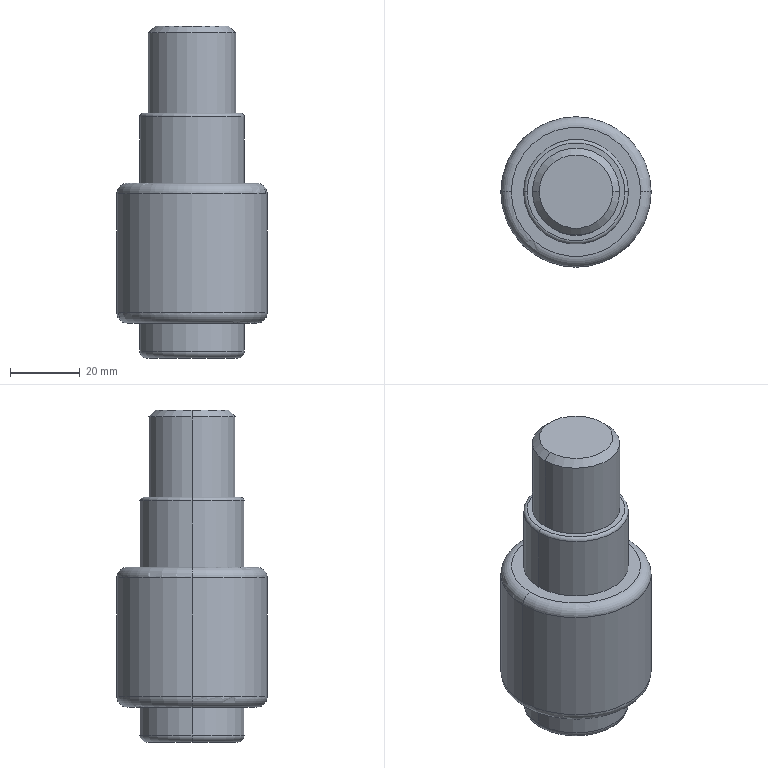Part | STEP file | Blocking air bag | 1 solid | 23 faces | box 43 x 43 x 95 mm | volume 90813 mm3 | torus 8 | cylinder 8 | plane 5 | cone 2 | commonest cylinder face diameters 30 x4 25 x2 43 x2
STEP:
#1=CARTESIAN_POINT('',(0.,0.,0.));
#2=DIRECTION('',(0.,0.,1.));
#3=DIRECTION('',(1.,0.,0.));
#4=AXIS2_PLACEMENT_3D('',#1,#2,#3);
#5=CARTESIAN_POINT('',(10.5,0.,95.));
#6=VERTEX_POINT('',#5);
#7=CARTESIAN_POINT('',(-10.5,0.,95.));
#8=VERTEX_POINT('',#7);
#9=CARTESIAN_POINT('',(0.,0.,95.));
#10=DIRECTION('',(0.,0.,1.));
#11=DIRECTION('',(1.,0.,0.));
#12=AXIS2_PLACEMENT_3D('',#9,#10,#11);
#13=CIRCLE('',#12,10.5);
#14=CARTESIAN_POINT('',(0.,0.,95.));
#15=DIRECTION('',(0.,0.,-1.));
#16=DIRECTION('',(-1.,0.,0.));
#17=AXIS2_PLACEMENT_3D('',#14,#15,#16);
#18=CONICAL_SURFACE('',#17,10.5,0.7854);
#19=CARTESIAN_POINT('',(3.142,0.));
#20=DIRECTION('',(-1.,0.));
#21=VECTOR('',#20,1.);
#22=LINE('',#19,#21);
#23=(GEOMETRIC_REPRESENTATION_CONTEXT(2)PARAMETRIC_REPRESENTATION_CONTEXT()REPRESENTATION_CONTEXT('',''));
#24=DEFINITIONAL_REPRESENTATION('',(#22),#23);
#25=PCURVE('',#18,#24);
#26=CARTESIAN_POINT('',(12.5,0.,95.));
#27=DIRECTION('',(0.,0.,1.));
#28=DIRECTION('',(1.,0.,0.));
#29=AXIS2_PLACEMENT_3D('',#26,#27,#28);
#30=PLANE('',#29);
#31=CARTESIAN_POINT('',(-12.5,0.));
#32=DIRECTION('',(1.,0.));
#33=AXIS2_PLACEMENT_2D('',#31,#32);
#34=CIRCLE('',#33,10.5);
#35=(GEOMETRIC_REPRESENTATION_CONTEXT(2)PARAMETRIC_REPRESENTATION_CONTEXT()REPRESENTATION_CONTEXT('',''));
#36=DEFINITIONAL_REPRESENTATION('',(#34),#35);
#37=PCURVE('',#30,#36);
#38=SURFACE_CURVE('',#13,(#25,#37),.PCURVE_S1.);
#39=EDGE_CURVE('',#6,#8,#38,.T.);
#40=ORIENTED_EDGE('',*,*,#39,.F.);
#41=CARTESIAN_POINT('',(12.5,0.,93.));
#42=VERTEX_POINT('',#41);
#43=CARTESIAN_POINT('',(10.5,0.,95.));
#44=DIRECTION('',(0.7071,0.,-0.7071));
#45=VECTOR('',#44,1.);
#46=LINE('',#43,#45);
#47=CARTESIAN_POINT('',(3.142,0.));
#48=DIRECTION('',(0.,1.));
#49=VECTOR('',#48,1.);
#50=LINE('',#47,#49);
#51=(GEOMETRIC_REPRESENTATION_CONTEXT(2)PARAMETRIC_REPRESENTATION_CONTEXT()REPRESENTATION_CONTEXT('',''));
#52=DEFINITIONAL_REPRESENTATION('',(#50),#51);
#53=PCURVE('',#18,#52);
#54=CARTESIAN_POINT('',(0.,0.,95.));
#55=DIRECTION('',(0.,0.,-1.));
#56=DIRECTION('',(-1.,0.,0.));
#57=AXIS2_PLACEMENT_3D('',#54,#55,#56);
#58=CONICAL_SURFACE('',#57,10.5,0.7854);
#59=CARTESIAN_POINT('',(3.142,0.));
#60=DIRECTION('',(0.,1.));
#61=VECTOR('',#60,1.);
#62=LINE('',#59,#61);
#63=(GEOMETRIC_REPRESENTATION_CONTEXT(2)PARAMETRIC_REPRESENTATION_CONTEXT()REPRESENTATION_CONTEXT('',''));
#64=DEFINITIONAL_REPRESENTATION('',(#62),#63);
#65=PCURVE('',#58,#64);
#66=SURFACE_CURVE('',#46,(#53,#65),.PCURVE_S1.);
#67=EDGE_CURVE('',#6,#42,#66,.T.);
#68=ORIENTED_EDGE('',*,*,#67,.T.);
#69=CARTESIAN_POINT('',(-12.5,0.,93.));
#70=VERTEX_POINT('',#69);
#71=CARTESIAN_POINT('',(0.,0.,93.));
#72=DIRECTION('',(0.,0.,-1.));
#73=DIRECTION('',(1.,0.,0.));
#74=AXIS2_PLACEMENT_3D('',#71,#72,#73);
#75=CIRCLE('',#74,12.5);
#76=CARTESIAN_POINT('',(-3.142,2.));
#77=DIRECTION('',(1.,0.));
#78=VECTOR('',#77,1.);
#79=LINE('',#76,#78);
#80=(GEOMETRIC_REPRESENTATION_CONTEXT(2)PARAMETRIC_REPRESENTATION_CONTEXT()REPRESENTATION_CONTEXT('',''));
#81=DEFINITIONAL_REPRESENTATION('',(#79),#80);
#82=PCURVE('',#18,#81);
#83=CARTESIAN_POINT('',(0.,0.,95.));
#84=DIRECTION('',(0.,0.,1.));
#85=DIRECTION('',(1.,0.,0.));
#86=AXIS2_PLACEMENT_3D('',#83,#84,#85);
#87=CYLINDRICAL_SURFACE('',#86,12.5);
#88=CARTESIAN_POINT('',(6.283,-2.));
#89=DIRECTION('',(-1.,0.));
#90=VECTOR('',#89,1.);
#91=LINE('',#88,#90);
#92=(GEOMETRIC_REPRESENTATION_CONTEXT(2)PARAMETRIC_REPRESENTATION_CONTEXT()REPRESENTATION_CONTEXT('',''));
#93=DEFINITIONAL_REPRESENTATION('',(#91),#92);
#94=PCURVE('',#87,#93);
#95=SURFACE_CURVE('',#75,(#82,#94),.PCURVE_S1.);
#96=EDGE_CURVE('',#70,#42,#95,.T.);
#97=ORIENTED_EDGE('',*,*,#96,.F.);
#98=CARTESIAN_POINT('',(-10.5,0.,95.));
#99=DIRECTION('',(-0.7071,0.,-0.7071));
#100=VECTOR('',#99,1.);
#101=LINE('',#98,#100);
#102=CARTESIAN_POINT('',(0.,0.));
#103=DIRECTION('',(0.,1.));
#104=VECTOR('',#103,1.);
#105=LINE('',#102,#104);
#106=(GEOMETRIC_REPRESENTATION_CONTEXT(2)PARAMETRIC_REPRESENTATION_CONTEXT()REPRESENTATION_CONTEXT('',''));
#107=DEFINITIONAL_REPRESENTATION('',(#105),#106);
#108=PCURVE('',#18,#107);
#109=CARTESIAN_POINT('',(6.283,0.));
#110=DIRECTION('',(0.,1.));
#111=VECTOR('',#110,1.);
#112=LINE('',#109,#111);
#113=(GEOMETRIC_REPRESENTATION_CONTEXT(2)PARAMETRIC_REPRESENTATION_CONTEXT()REPRESENTATION_CONTEXT('',''));
#114=DEFINITIONAL_REPRESENTATION('',(#112),#113);
#115=PCURVE('',#58,#114);
#116=SURFACE_CURVE('',#101,(#108,#115),.PCURVE_S1.);
#117=EDGE_CURVE('',#8,#70,#116,.T.);
#118=ORIENTED_EDGE('',*,*,#117,.F.);
#119=EDGE_LOOP('',(#40,#68,#97,#118));
#120=FACE_BOUND('',#119,.T.);
#121=ADVANCED_FACE('',(#120),#18,.T.);
#122=CARTESIAN_POINT('',(15.,0.,2.));
#123=VERTEX_POINT('',#122);
#124=CARTESIAN_POINT('',(-15.,0.,2.));
#125=VERTEX_POINT('',#124);
#126=CARTESIAN_POINT('',(0.,0.,2.));
#127=DIRECTION('',(0.,0.,1.));
#128=DIRECTION('',(-1.,0.,0.));
#129=AXIS2_PLACEMENT_3D('',#126,#127,#128);
#130=CIRCLE('',#129,15.);
#131=CARTESIAN_POINT('',(0.,0.,2.));
#132=DIRECTION('',(0.,0.,-1.));
#133=DIRECTION('',(-1.,0.,0.));
#134=AXIS2_PLACEMENT_3D('',#131,#132,#133);
#135=TOROIDAL_SURFACE('',#134,13.,2.);
#136=CARTESIAN_POINT('',(6.283,0.));
#137=DIRECTION('',(-1.,0.));
#138=VECTOR('',#137,1.);
#139=LINE('',#136,#138);
#140=(GEOMETRIC_REPRESENTATION_CONTEXT(2)PARAMETRIC_REPRESENTATION_CONTEXT()REPRESENTATION_CONTEXT('',''));
#141=DEFINITIONAL_REPRESENTATION('',(#139),#140);
#142=PCURVE('',#135,#141);
#143=CARTESIAN_POINT('',(0.,0.,95.));
#144=DIRECTION('',(0.,0.,1.));
#145=DIRECTION('',(1.,0.,0.));
#146=AXIS2_PLACEMENT_3D('',#143,#144,#145);
#147=CYLINDRICAL_SURFACE('',#146,15.);
#148=CARTESIAN_POINT('',(-3.142,-93.));
#149=DIRECTION('',(1.,0.));
#150=VECTOR('',#149,1.);
#151=LINE('',#148,#150);
#152=(GEOMETRIC_REPRESENTATION_CONTEXT(2)PARAMETRIC_REPRESENTATION_CONTEXT()REPRESENTATION_CONTEXT('',''));
#153=DEFINITIONAL_REPRESENTATION('',(#151),#152);
#154=PCURVE('',#147,#153);
#155=SURFACE_CURVE('',#130,(#142,#154),.PCURVE_S1.);
#156=EDGE_CURVE('',#123,#125,#155,.T.);
#157=ORIENTED_EDGE('',*,*,#156,.F.);
#158=CARTESIAN_POINT('',(13.,0.,0.));
#159=VERTEX_POINT('',#158);
#160=CARTESIAN_POINT('',(13.,0.,2.));
#161=DIRECTION('',(0.,1.,0.));
#162=DIRECTION('',(-1.,0.,0.));
#163=AXIS2_PLACEMENT_3D('',#160,#161,#162);
#164=CIRCLE('',#163,2.);
#165=CARTESIAN_POINT('',(3.142,-3.142));
#166=DIRECTION('',(0.,1.));
#167=VECTOR('',#166,1.);
#168=LINE('',#165,#167);
#169=(GEOMETRIC_REPRESENTATION_CONTEXT(2)PARAMETRIC_REPRESENTATION_CONTEXT()REPRESENTATION_CONTEXT('',''));
#170=DEFINITIONAL_REPRESENTATION('',(#168),#169);
#171=PCURVE('',#135,#170);
#172=CARTESIAN_POINT('',(0.,0.,2.));
#173=DIRECTION('',(0.,0.,-1.));
#174=DIRECTION('',(-1.,0.,0.));
#175=AXIS2_PLACEMENT_3D('',#172,#173,#174);
#176=TOROIDAL_SURFACE('',#175,13.,2.);
#177=CARTESIAN_POINT('',(3.142,-3.142));
#178=DIRECTION('',(0.,1.));
#179=VECTOR('',#178,1.);
#180=LINE('',#177,#179);
#181=(GEOMETRIC_REPRESENTATION_CONTEXT(2)PARAMETRIC_REPRESENTATION_CONTEXT()REPRESENTATION_CONTEXT('',''));
#182=DEFINITIONAL_REPRESENTATION('',(#180),#181);
#183=PCURVE('',#176,#182);
#184=SURFACE_CURVE('',#164,(#171,#183),.PCURVE_S1.);
#185=EDGE_CURVE('',#123,#159,#184,.T.);
#186=ORIENTED_EDGE('',*,*,#185,.T.);
#187=CARTESIAN_POINT('',(-13.,0.,0.));
#188=VERTEX_POINT('',#187);
#189=CARTESIAN_POINT('',(0.,0.,0.));
#190=DIRECTION('',(0.,0.,-1.));
#191=DIRECTION('',(-1.,0.,0.));
#192=AXIS2_PLACEMENT_3D('',#189,#190,#191);
#193=CIRCLE('',#192,13.);
#194=CARTESIAN_POINT('',(0.,1.571));
#195=DIRECTION('',(1.,0.));
#196=VECTOR('',#195,1.);
#197=LINE('',#194,#196);
#198=(GEOMETRIC_REPRESENTATION_CONTEXT(2)PARAMETRIC_REPRESENTATION_CONTEXT()REPRESENTATION_CONTEXT('',''));
#199=DEFINITIONAL_REPRESENTATION('',(#197),#198);
#200=PCURVE('',#135,#199);
#201=CARTESIAN_POINT('',(0.,0.,0.));
#202=DIRECTION('',(0.,0.,-1.));
#203=DIRECTION('',(-1.,0.,0.));
#204=AXIS2_PLACEMENT_3D('',#201,#202,#203);
#205=PLANE('',#204);
#206=CARTESIAN_POINT('',(0.,0.));
#207=DIRECTION('',(1.,0.));
#208=AXIS2_PLACEMENT_2D('',#206,#207);
#209=CIRCLE('',#208,13.);
#210=(GEOMETRIC_REPRESENTATION_CONTEXT(2)PARAMETRIC_REPRESENTATION_CONTEXT()REPRESENTATION_CONTEXT('',''));
#211=DEFINITIONAL_REPRESENTATION('',(#209),#210);
#212=PCURVE('',#205,#211);
#213=SURFACE_CURVE('',#193,(#200,#212),.PCURVE_S1.);
#214=EDGE_CURVE('',#188,#159,#213,.T.);
#215=ORIENTED_EDGE('',*,*,#214,.F.);
#216=CARTESIAN_POINT('',(-13.,0.,2.));
#217=DIRECTION('',(0.,-1.,0.));
#218=DIRECTION('',(0.,0.,-1.));
#219=AXIS2_PLACEMENT_3D('',#216,#217,#218);
#220=CIRCLE('',#219,2.);
#221=CARTESIAN_POINT('',(0.,-4.712));
#222=DIRECTION('',(0.,1.));
#223=VECTOR('',#222,1.);
#224=LINE('',#221,#223);
#225=(GEOMETRIC_REPRESENTATION_CONTEXT(2)PARAMETRIC_REPRESENTATION_CONTEXT()REPRESENTATION_CONTEXT('',''));
#226=DEFINITIONAL_REPRESENTATION('',(#224),#225);
#227=PCURVE('',#135,#226);
#228=CARTESIAN_POINT('',(6.283,-4.712));
#229=DIRECTION('',(0.,1.));
#230=VECTOR('',#229,1.);
#231=LINE('',#228,#230);
#232=(GEOMETRIC_REPRESENTATION_CONTEXT(2)PARAMETRIC_REPRESENTATION_CONTEXT()REPRESENTATION_CONTEXT('',''));
#233=DEFINITIONAL_REPRESENTATION('',(#231),#232);
#234=PCURVE('',#176,#233);
#235=SURFACE_CURVE('',#220,(#227,#234),.PCURVE_S1.);
#236=EDGE_CURVE('',#125,#188,#235,.T.);
#237=ORIENTED_EDGE('',*,*,#236,.F.);
#238=EDGE_LOOP('',(#157,#186,#215,#237));
#239=FACE_BOUND('',#238,.T.);
#240=ADVANCED_FACE('',(#239),#135,.T.);
#241=CARTESIAN_POINT('',(-15.,0.,69.));
#242=VERTEX_POINT('',#241);
#243=CARTESIAN_POINT('',(15.,0.,69.));
#244=VERTEX_POINT('',#243);
#245=CARTESIAN_POINT('',(0.,0.,69.));
#246=DIRECTION('',(0.,0.,-1.));
#247=DIRECTION('',(1.,0.,0.));
#248=AXIS2_PLACEMENT_3D('',#245,#246,#247);
#249=CIRCLE('',#248,15.);
#250=CARTESIAN_POINT('',(0.,0.,69.));
#251=DIRECTION('',(0.,0.,1.));
#252=DIRECTION('',(1.,0.,0.));
#253=AXIS2_PLACEMENT_3D('',#250,#251,#252);
#254=TOROIDAL_SURFACE('',#253,14.,1.);
#255=CARTESIAN_POINT('',(6.283,0.));
#256=DIRECTION('',(-1.,0.));
#257=VECTOR('',#256,1.);
#258=LINE('',#255,#257);
#259=(GEOMETRIC_REPRESENTATION_CONTEXT(2)PARAMETRIC_REPRESENTATION_CONTEXT()REPRESENTATION_CONTEXT('',''));
#260=DEFINITIONAL_REPRESENTATION('',(#258),#259);
#261=PCURVE('',#254,#260);
#262=CARTESIAN_POINT('',(0.,0.,95.));
#263=DIRECTION('',(0.,0.,1.));
#264=DIRECTION('',(1.,0.,0.));
#265=AXIS2_PLACEMENT_3D('',#262,#263,#264);
#266=CYLINDRICAL_SURFACE('',#265,15.);
#267=CARTESIAN_POINT('',(6.283,-26.));
#268=DIRECTION('',(-1.,0.));
#269=VECTOR('',#268,1.);
#270=LINE('',#267,#269);
#271=(GEOMETRIC_REPRESENTATION_CONTEXT(2)PARAMETRIC_REPRESENTATION_CONTEXT()REPRESENTATION_CONTEXT('',''));
#272=DEFINITIONAL_REPRESENTATION('',(#270),#271);
#273=PCURVE('',#266,#272);
#274=SURFACE_CURVE('',#249,(#261,#273),.PCURVE_S1.);
#275=EDGE_CURVE('',#242,#244,#274,.T.);
#276=ORIENTED_EDGE('',*,*,#275,.F.);
#277=CARTESIAN_POINT('',(-14.,0.,70.));
#278=VERTEX_POINT('',#277);
#279=CARTESIAN_POINT('',(-14.,0.,69.));
#280=DIRECTION('',(0.,1.,0.));
#281=DIRECTION('',(-1.,0.,0.));
#282=AXIS2_PLACEMENT_3D('',#279,#280,#281);
#283=CIRCLE('',#282,1.);
#284=CARTESIAN_POINT('',(3.142,0.));
#285=DIRECTION('',(0.,1.));
#286=VECTOR('',#285,1.);
#287=LINE('',#284,#286);
#288=(GEOMETRIC_REPRESENTATION_CONTEXT(2)PARAMETRIC_REPRESENTATION_CONTEXT()REPRESENTATION_CONTEXT('',''));
#289=DEFINITIONAL_REPRESENTATION('',(#287),#288);
#290=PCURVE('',#254,#289);
#291=CARTESIAN_POINT('',(0.,0.,69.));
#292=DIRECTION('',(0.,0.,1.));
#293=DIRECTION('',(1.,0.,0.));
#294=AXIS2_PLACEMENT_3D('',#291,#292,#293);
#295=TOROIDAL_SURFACE('',#294,14.,1.);
#296=CARTESIAN_POINT('',(3.142,0.));
#297=DIRECTION('',(0.,1.));
#298=VECTOR('',#297,1.);
#299=LINE('',#296,#298);
#300=(GEOMETRIC_REPRESENTATION_CONTEXT(2)PARAMETRIC_REPRESENTATION_CONTEXT()REPRESENTATION_CONTEXT('',''));
#301=DEFINITIONAL_REPRESENTATION('',(#299),#300);
#302=PCURVE('',#295,#301);
#303=SURFACE_CURVE('',#283,(#290,#302),.PCURVE_S1.);
#304=EDGE_CURVE('',#242,#278,#303,.T.);
#305=ORIENTED_EDGE('',*,*,#304,.T.);
#306=CARTESIAN_POINT('',(14.,0.,70.));
#307=VERTEX_POINT('',#306);
#308=CARTESIAN_POINT('',(0.,0.,70.));
#309=DIRECTION('',(0.,0.,1.));
#310=DIRECTION('',(1.,0.,0.));
#311=AXIS2_PLACEMENT_3D('',#308,#309,#310);
#312=CIRCLE('',#311,14.);
#313=CARTESIAN_POINT('',(0.,1.571));
#314=DIRECTION('',(1.,0.));
#315=VECTOR('',#314,1.);
#316=LINE('',#313,#315);
#317=(GEOMETRIC_REPRESENTATION_CONTEXT(2)PARAMETRIC_REPRESENTATION_CONTEXT()REPRESENTATION_CONTEXT('',''));
#318=DEFINITIONAL_REPRESENTATION('',(#316),#317);
#319=PCURVE('',#254,#318);
#320=CARTESIAN_POINT('',(15.,0.,70.));
#321=DIRECTION('',(0.,0.,1.));
#322=DIRECTION('',(1.,0.,0.));
#323=AXIS2_PLACEMENT_3D('',#320,#321,#322);
#324=PLANE('',#323);
#325=CARTESIAN_POINT('',(-15.,0.));
#326=DIRECTION('',(1.,0.));
#327=AXIS2_PLACEMENT_2D('',#325,#326);
#328=CIRCLE('',#327,14.);
#329=(GEOMETRIC_REPRESENTATION_CONTEXT(2)PARAMETRIC_REPRESENTATION_CONTEXT()REPRESENTATION_CONTEXT('',''));
#330=DEFINITIONAL_REPRESENTATION('',(#328),#329);
#331=PCURVE('',#324,#330);
#332=SURFACE_CURVE('',#312,(#319,#331),.PCURVE_S1.);
#333=EDGE_CURVE('',#307,#278,#332,.T.);
#334=ORIENTED_EDGE('',*,*,#333,.F.);
#335=CARTESIAN_POINT('',(14.,0.,69.));
#336=DIRECTION('',(0.,-1.,0.));
#337=DIRECTION('',(0.,0.,-1.));
#338=AXIS2_PLACEMENT_3D('',#335,#336,#337);
#339=CIRCLE('',#338,1.);
#340=CARTESIAN_POINT('',(0.,-1.571));
#341=DIRECTION('',(0.,1.));
#342=VECTOR('',#341,1.);
#343=LINE('',#340,#342);
#344=(GEOMETRIC_REPRESENTATION_CONTEXT(2)PARAMETRIC_REPRESENTATION_CONTEXT()REPRESENTATION_CONTEXT('',''));
#345=DEFINITIONAL_REPRESENTATION('',(#343),#344);
#346=PCURVE('',#254,#345);
#347=CARTESIAN_POINT('',(6.283,-1.571));
#348=DIRECTION('',(0.,1.));
#349=VECTOR('',#348,1.);
#350=LINE('',#347,#349);
#351=(GEOMETRIC_REPRESENTATION_CONTEXT(2)PARAMETRIC_REPRESENTATION_CONTEXT()REPRESENTATION_CONTEXT('',''));
#352=DEFINITIONAL_REPRESENTATION('',(#350),#351);
#353=PCURVE('',#295,#352);
#354=SURFACE_CURVE('',#339,(#346,#353),.PCURVE_S1.);
#355=EDGE_CURVE('',#244,#307,#354,.T.);
#356=ORIENTED_EDGE('',*,*,#355,.F.);
#357=EDGE_LOOP('',(#276,#305,#334,#356));
#358=FACE_BOUND('',#357,.T.);
#359=ADVANCED_FACE('',(#358),#254,.T.);
#360=CARTESIAN_POINT('',(21.5,0.,13.));
#361=VERTEX_POINT('',#360);
#362=CARTESIAN_POINT('',(-21.5,0.,13.));
#363=VERTEX_POINT('',#362);
#364=CARTESIAN_POINT('',(0.,0.,13.));
#365=DIRECTION('',(0.,0.,1.));
#366=DIRECTION('',(-1.,0.,0.));
#367=AXIS2_PLACEMENT_3D('',#364,#365,#366);
#368=CIRCLE('',#367,21.5);
#369=CARTESIAN_POINT('',(0.,0.,13.));
#370=DIRECTION('',(0.,0.,-1.));
#371=DIRECTION('',(-1.,0.,0.));
#372=AXIS2_PLACEMENT_3D('',#369,#370,#371);
#373=TOROIDAL_SURFACE('',#372,18.5,3.);
#374=CARTESIAN_POINT('',(6.283,0.));
#375=DIRECTION('',(-1.,0.));
#376=VECTOR('',#375,1.);
#377=LINE('',#374,#376);
#378=(GEOMETRIC_REPRESENTATION_CONTEXT(2)PARAMETRIC_REPRESENTATION_CONTEXT()REPRESENTATION_CONTEXT('',''));
#379=DEFINITIONAL_REPRESENTATION('',(#377),#378);
#380=PCURVE('',#373,#379);
#381=CARTESIAN_POINT('',(0.,0.,95.));
#382=DIRECTION('',(0.,0.,1.));
#383=DIRECTION('',(1.,0.,0.));
#384=AXIS2_PLACEMENT_3D('',#381,#382,#383);
#385=CYLINDRICAL_SURFACE('',#384,21.5);
#386=CARTESIAN_POINT('',(-3.142,-82.));
#387=DIRECTION('',(1.,0.));
#388=VECTOR('',#387,1.);
#389=LINE('',#386,#388);
#390=(GEOMETRIC_REPRESENTATION_CONTEXT(2)PARAMETRIC_REPRESENTATION_CONTEXT()REPRESENTATION_CONTEXT('',''));
#391=DEFINITIONAL_REPRESENTATION('',(#389),#390);
#392=PCURVE('',#385,#391);
#393=SURFACE_CURVE('',#368,(#380,#392),.PCURVE_S1.);
#394=EDGE_CURVE('',#361,#363,#393,.T.);
#395=ORIENTED_EDGE('',*,*,#394,.F.);
#396=CARTESIAN_POINT('',(18.5,0.,10.));
#397=VERTEX_POINT('',#396);
#398=CARTESIAN_POINT('',(18.5,0.,13.));
#399=DIRECTION('',(0.,1.,0.));
#400=DIRECTION('',(-1.,0.,0.));
#401=AXIS2_PLACEMENT_3D('',#398,#399,#400);
#402=CIRCLE('',#401,3.);
#403=CARTESIAN_POINT('',(3.142,-3.142));
#404=DIRECTION('',(0.,1.));
#405=VECTOR('',#404,1.);
#406=LINE('',#403,#405);
#407=(GEOMETRIC_REPRESENTATION_CONTEXT(2)PARAMETRIC_REPRESENTATION_CONTEXT()REPRESENTATION_CONTEXT('',''));
#408=DEFINITIONAL_REPRESENTATION('',(#406),#407);
#409=PCURVE('',#373,#408);
#410=CARTESIAN_POINT('',(0.,0.,13.));
#411=DIRECTION('',(0.,0.,-1.));
#412=DIRECTION('',(-1.,0.,0.));
#413=AXIS2_PLACEMENT_3D('',#410,#411,#412);
#414=TOROIDAL_SURFACE('',#413,18.5,3.);
#415=CARTESIAN_POINT('',(3.142,-3.142));
#416=DIRECTION('',(0.,1.));
#417=VECTOR('',#416,1.);
#418=LINE('',#415,#417);
#419=(GEOMETRIC_REPRESENTATION_CONTEXT(2)PARAMETRIC_REPRESENTATION_CONTEXT()REPRESENTATION_CONTEXT('',''));
#420=DEFINITIONAL_REPRESENTATION('',(#418),#419);
#421=PCURVE('',#414,#420);
#422=SURFACE_CURVE('',#402,(#409,#421),.PCURVE_S1.);
#423=EDGE_CURVE('',#361,#397,#422,.T.);
#424=ORIENTED_EDGE('',*,*,#423,.T.);
#425=CARTESIAN_POINT('',(-18.5,0.,10.));
#426=VERTEX_POINT('',#425);
#427=CARTESIAN_POINT('',(0.,0.,10.));
#428=DIRECTION('',(0.,0.,-1.));
#429=DIRECTION('',(-1.,0.,0.));
#430=AXIS2_PLACEMENT_3D('',#427,#428,#429);
#431=CIRCLE('',#430,18.5);
#432=CARTESIAN_POINT('',(0.,1.571));
#433=DIRECTION('',(1.,0.));
#434=VECTOR('',#433,1.);
#435=LINE('',#432,#434);
#436=(GEOMETRIC_REPRESENTATION_CONTEXT(2)PARAMETRIC_REPRESENTATION_CONTEXT()REPRESENTATION_CONTEXT('',''));
#437=DEFINITIONAL_REPRESENTATION('',(#435),#436);
#438=PCURVE('',#373,#437);
#439=CARTESIAN_POINT('',(15.,0.,10.));
#440=DIRECTION('',(0.,0.,-1.));
#441=DIRECTION('',(-1.,0.,0.));
#442=AXIS2_PLACEMENT_3D('',#439,#440,#441);
#443=PLANE('',#442);
#444=CARTESIAN_POINT('',(15.,0.));
#445=DIRECTION('',(1.,0.));
#446=AXIS2_PLACEMENT_2D('',#444,#445);
#447=CIRCLE('',#446,18.5);
#448=(GEOMETRIC_REPRESENTATION_CONTEXT(2)PARAMETRIC_REPRESENTATION_CONTEXT()REPRESENTATION_CONTEXT('',''));
#449=DEFINITIONAL_REPRESENTATION('',(#447),#448);
#450=PCURVE('',#443,#449);
#451=SURFACE_CURVE('',#431,(#438,#450),.PCURVE_S1.);
#452=EDGE_CURVE('',#426,#397,#451,.T.);
#453=ORIENTED_EDGE('',*,*,#452,.F.);
#454=CARTESIAN_POINT('',(-18.5,0.,13.));
#455=DIRECTION('',(0.,-1.,0.));
#456=DIRECTION('',(0.,0.,-1.));
#457=AXIS2_PLACEMENT_3D('',#454,#455,#456);
#458=CIRCLE('',#457,3.);
#459=CARTESIAN_POINT('',(0.,-4.712));
#460=DIRECTION('',(0.,1.));
#461=VECTOR('',#460,1.);
#462=LINE('',#459,#461);
#463=(GEOMETRIC_REPRESENTATION_CONTEXT(2)PARAMETRIC_REPRESENTATION_CONTEXT()REPRESENTATION_CONTEXT('',''));
#464=DEFINITIONAL_REPRESENTATION('',(#462),#463);
#465=PCURVE('',#373,#464);
#466=CARTESIAN_POINT('',(6.283,-4.712));
#467=DIRECTION('',(0.,1.));
#468=VECTOR('',#467,1.);
#469=LINE('',#466,#468);
#470=(GEOMETRIC_REPRESENTATION_CONTEXT(2)PARAMETRIC_REPRESENTATION_CONTEXT()REPRESENTATION_CONTEXT('',''));
#471=DEFINITIONAL_REPRESENTATION('',(#469),#470);
#472=PCURVE('',#414,#471);
#473=SURFACE_CURVE('',#458,(#465,#472),.PCURVE_S1.);
#474=EDGE_CURVE('',#363,#426,#473,.T.);
#475=ORIENTED_EDGE('',*,*,#474,.F.);
#476=EDGE_LOOP('',(#395,#424,#453,#475));
#477=FACE_BOUND('',#476,.T.);
#478=ADVANCED_FACE('',(#477),#373,.T.);
#479=CARTESIAN_POINT('',(-21.5,0.,47.));
#480=VERTEX_POINT('',#479);
#481=CARTESIAN_POINT('',(21.5,0.,47.));
#482=VERTEX_POINT('',#481);
#483=CARTESIAN_POINT('',(0.,0.,47.));
#484=DIRECTION('',(0.,0.,-1.));
#485=DIRECTION('',(1.,0.,0.));
#486=AXIS2_PLACEMENT_3D('',#483,#484,#485);
#487=CIRCLE('',#486,21.5);
#488=CARTESIAN_POINT('',(0.,0.,47.));
#489=DIRECTION('',(0.,0.,1.));
#490=DIRECTION('',(1.,0.,0.));
#491=AXIS2_PLACEMENT_3D('',#488,#489,#490);
#492=TOROIDAL_SURFACE('',#491,18.5,3.);
#493=CARTESIAN_POINT('',(6.283,0.));
#494=DIRECTION('',(-1.,0.));
#495=VECTOR('',#494,1.);
#496=LINE('',#493,#495);
#497=(GEOMETRIC_REPRESENTATION_CONTEXT(2)PARAMETRIC_REPRESENTATION_CONTEXT()REPRESENTATION_CONTEXT('',''));
#498=DEFINITIONAL_REPRESENTATION('',(#496),#497);
#499=PCURVE('',#492,#498);
#500=CARTESIAN_POINT('',(6.283,-48.));
#501=DIRECTION('',(-1.,0.));
#502=VECTOR('',#501,1.);
#503=LINE('',#500,#502);
#504=(GEOMETRIC_REPRESENTATION_CONTEXT(2)PARAMETRIC_REPRESENTATION_CONTEXT()REPRESENTATION_CONTEXT('',''));
#505=DEFINITIONAL_REPRESENTATION('',(#503),#504);
#506=PCURVE('',#385,#505);
#507=SURFACE_CURVE('',#487,(#499,#506),.PCURVE_S1.);
#508=EDGE_CURVE('',#480,#482,#507,.T.);
#509=ORIENTED_EDGE('',*,*,#508,.F.);
#510=CARTESIAN_POINT('',(-18.5,0.,50.));
#511=VERTEX_POINT('',#510);
#512=CARTESIAN_POINT('',(-18.5,0.,47.));
#513=DIRECTION('',(0.,1.,0.));
#514=DIRECTION('',(-1.,0.,0.));
#515=AXIS2_PLACEMENT_3D('',#512,#513,#514);
#516=CIRCLE('',#515,3.);
#517=CARTESIAN_POINT('',(3.142,0.));
#518=DIRECTION('',(0.,1.));
#519=VECTOR('',#518,1.);
#520=LINE('',#517,#519);
#521=(GEOMETRIC_REPRESENTATION_CONTEXT(2)PARAMETRIC_REPRESENTATION_CONTEXT()REPRESENTATION_CONTEXT('',''));
#522=DEFINITIONAL_REPRESENTATION('',(#520),#521);
#523=PCURVE('',#492,#522);
#524=CARTESIAN_POINT('',(0.,0.,47.));
#525=DIRECTION('',(0.,0.,1.));
#526=DIRECTION('',(1.,0.,0.));
#527=AXIS2_PLACEMENT_3D('',#524,#525,#526);
#528=TOROIDAL_SURFACE('',#527,18.5,3.);
#529=CARTESIAN_POINT('',(3.142,0.));
#530=DIRECTION('',(0.,1.));
#531=VECTOR('',#530,1.);
#532=LINE('',#529,#531);
#533=(GEOMETRIC_REPRESENTATION_CONTEXT(2)PARAMETRIC_REPRESENTATION_CONTEXT()REPRESENTATION_CONTEXT('',''));
#534=DEFINITIONAL_REPRESENTATION('',(#532),#533);
#535=PCURVE('',#528,#534);
#536=SURFACE_CURVE('',#516,(#523,#535),.PCURVE_S1.);
#537=EDGE_CURVE('',#480,#511,#536,.T.);
#538=ORIENTED_EDGE('',*,*,#537,.T.);
#539=CARTESIAN_POINT('',(18.5,0.,50.));
#540=VERTEX_POINT('',#539);
#541=CARTESIAN_POINT('',(0.,0.,50.));
#542=DIRECTION('',(0.,0.,1.));
#543=DIRECTION('',(1.,0.,0.));
#544=AXIS2_PLACEMENT_3D('',#541,#542,#543);
#545=CIRCLE('',#544,18.5);
#546=CARTESIAN_POINT('',(0.,1.571));
#547=DIRECTION('',(1.,0.));
#548=VECTOR('',#547,1.);
#549=LINE('',#546,#548);
#550=(GEOMETRIC_REPRESENTATION_CONTEXT(2)PARAMETRIC_REPRESENTATION_CONTEXT()REPRESENTATION_CONTEXT('',''));
#551=DEFINITIONAL_REPRESENTATION('',(#549),#550);
#552=PCURVE('',#492,#551);
#553=CARTESIAN_POINT('',(15.,0.,50.));
#554=DIRECTION('',(0.,0.,1.));
#555=DIRECTION('',(1.,0.,0.));
#556=AXIS2_PLACEMENT_3D('',#553,#554,#555);
#557=PLANE('',#556);
#558=CARTESIAN_POINT('',(-15.,0.));
#559=DIRECTION('',(1.,0.));
#560=AXIS2_PLACEMENT_2D('',#558,#559);
#561=CIRCLE('',#560,18.5);
#562=(GEOMETRIC_REPRESENTATION_CONTEXT(2)PARAMETRIC_REPRESENTATION_CONTEXT()REPRESENTATION_CONTEXT('',''));
#563=DEFINITIONAL_REPRESENTATION('',(#561),#562);
#564=PCURVE('',#557,#563);
#565=SURFACE_CURVE('',#545,(#552,#564),.PCURVE_S1.);
#566=EDGE_CURVE('',#540,#511,#565,.T.);
#567=ORIENTED_EDGE('',*,*,#566,.F.);
#568=CARTESIAN_POINT('',(18.5,0.,47.));
#569=DIRECTION('',(0.,-1.,0.));
#570=DIRECTION('',(0.,0.,-1.));
#571=AXIS2_PLACEMENT_3D('',#568,#569,#570);
#572=CIRCLE('',#571,3.);
#573=CARTESIAN_POINT('',(0.,-1.571));
#574=DIRECTION('',(0.,1.));
#575=VECTOR('',#574,1.);
#576=LINE('',#573,#575);
#577=(GEOMETRIC_REPRESENTATION_CONTEXT(2)PARAMETRIC_REPRESENTATION_CONTEXT()REPRESENTATION_CONTEXT('',''));
#578=DEFINITIONAL_REPRESENTATION('',(#576),#577);
#579=PCURVE('',#492,#578);
#580=CARTESIAN_POINT('',(6.283,-1.571));
#581=DIRECTION('',(0.,1.));
#582=VECTOR('',#581,1.);
#583=LINE('',#580,#582);
#584=(GEOMETRIC_REPRESENTATION_CONTEXT(2)PARAMETRIC_REPRESENTATION_CONTEXT()REPRESENTATION_CONTEXT('',''));
#585=DEFINITIONAL_REPRESENTATION('',(#583),#584);
#586=PCURVE('',#528,#585);
#587=SURFACE_CURVE('',#572,(#579,#586),.PCURVE_S1.);
#588=EDGE_CURVE('',#482,#540,#587,.T.);
#589=ORIENTED_EDGE('',*,*,#588,.F.);
#590=EDGE_LOOP('',(#509,#538,#567,#589));
#591=FACE_BOUND('',#590,.T.);
#592=ADVANCED_FACE('',(#591),#492,.T.);
#593=CARTESIAN_POINT('',(12.5,0.,70.));
#594=VERTEX_POINT('',#593);
#595=CARTESIAN_POINT('',(-12.5,0.,70.));
#596=VERTEX_POINT('',#595);
#597=CARTESIAN_POINT('',(0.,0.,70.));
#598=DIRECTION('',(0.,0.,1.));
#599=DIRECTION('',(1.,0.,0.));
#600=AXIS2_PLACEMENT_3D('',#597,#598,#599);
#601=CIRCLE('',#600,12.5);
#602=CARTESIAN_POINT('',(0.,-25.));
#603=DIRECTION('',(1.,0.));
#604=VECTOR('',#603,1.);
#605=LINE('',#602,#604);
#606=(GEOMETRIC_REPRESENTATION_CONTEXT(2)PARAMETRIC_REPRESENTATION_CONTEXT()REPRESENTATION_CONTEXT('',''));
#607=DEFINITIONAL_REPRESENTATION('',(#605),#606);
#608=PCURVE('',#87,#607);
#609=CARTESIAN_POINT('',(-15.,0.));
#610=DIRECTION('',(1.,0.));
#611=AXIS2_PLACEMENT_2D('',#609,#610);
#612=CIRCLE('',#611,12.5);
#613=(GEOMETRIC_REPRESENTATION_CONTEXT(2)PARAMETRIC_REPRESENTATION_CONTEXT()REPRESENTATION_CONTEXT('',''));
#614=DEFINITIONAL_REPRESENTATION('',(#612),#613);
#615=PCURVE('',#324,#614);
#616=SURFACE_CURVE('',#601,(#608,#615),.PCURVE_S1.);
#617=EDGE_CURVE('',#594,#596,#616,.T.);
#618=ORIENTED_EDGE('',*,*,#617,.T.);
#619=CARTESIAN_POINT('',(-12.5,0.,95.));
#620=DIRECTION('',(0.,0.,1.));
#621=VECTOR('',#620,1.);
#622=LINE('',#619,#621);
#623=CARTESIAN_POINT('',(3.142,0.));
#624=DIRECTION('',(0.,1.));
#625=VECTOR('',#624,1.);
#626=LINE('',#623,#625);
#627=(GEOMETRIC_REPRESENTATION_CONTEXT(2)PARAMETRIC_REPRESENTATION_CONTEXT()REPRESENTATION_CONTEXT('',''));
#628=DEFINITIONAL_REPRESENTATION('',(#626),#627);
#629=PCURVE('',#87,#628);
#630=CARTESIAN_POINT('',(0.,0.,95.));
#631=DIRECTION('',(0.,0.,1.));
#632=DIRECTION('',(1.,0.,0.));
#633=AXIS2_PLACEMENT_3D('',#630,#631,#632);
#634=CYLINDRICAL_SURFACE('',#633,12.5);
#635=CARTESIAN_POINT('',(3.142,0.));
#636=DIRECTION('',(0.,1.));
#637=VECTOR('',#636,1.);
#638=LINE('',#635,#637);
#639=(GEOMETRIC_REPRESENTATION_CONTEXT(2)PARAMETRIC_REPRESENTATION_CONTEXT()REPRESENTATION_CONTEXT('',''));
#640=DEFINITIONAL_REPRESENTATION('',(#638),#639);
#641=PCURVE('',#634,#640);
#642=SURFACE_CURVE('',#622,(#629,#641),.PCURVE_S1.);
#643=EDGE_CURVE('',#596,#70,#642,.T.);
#644=ORIENTED_EDGE('',*,*,#643,.T.);
#645=ORIENTED_EDGE('',*,*,#96,.T.);
#646=CARTESIAN_POINT('',(12.5,0.,95.));
#647=DIRECTION('',(0.,0.,1.));
#648=VECTOR('',#647,1.);
#649=LINE('',#646,#648);
#650=CARTESIAN_POINT('',(0.,0.));
#651=DIRECTION('',(0.,1.));
#652=VECTOR('',#651,1.);
#653=LINE('',#650,#652);
#654=(GEOMETRIC_REPRESENTATION_CONTEXT(2)PARAMETRIC_REPRESENTATION_CONTEXT()REPRESENTATION_CONTEXT('',''));
#655=DEFINITIONAL_REPRESENTATION('',(#653),#654);
#656=PCURVE('',#87,#655);
#657=CARTESIAN_POINT('',(6.283,0.));
#658=DIRECTION('',(0.,1.));
#659=VECTOR('',#658,1.);
#660=LINE('',#657,#659);
#661=(GEOMETRIC_REPRESENTATION_CONTEXT(2)PARAMETRIC_REPRESENTATION_CONTEXT()REPRESENTATION_CONTEXT('',''));
#662=DEFINITIONAL_REPRESENTATION('',(#660),#661);
#663=PCURVE('',#634,#662);
#664=SURFACE_CURVE('',#649,(#656,#663),.PCURVE_S1.);
#665=EDGE_CURVE('',#594,#42,#664,.T.);
#666=ORIENTED_EDGE('',*,*,#665,.F.);
#667=EDGE_LOOP('',(#618,#644,#645,#666));
#668=FACE_BOUND('',#667,.T.);
#669=ADVANCED_FACE('',(#668),#87,.T.);
#670=CARTESIAN_POINT('',(15.,0.,50.));
#671=VERTEX_POINT('',#670);
#672=CARTESIAN_POINT('',(-15.,0.,50.));
#673=VERTEX_POINT('',#672);
#674=CARTESIAN_POINT('',(0.,0.,50.));
#675=DIRECTION('',(0.,0.,1.));
#676=DIRECTION('',(1.,0.,0.));
#677=AXIS2_PLACEMENT_3D('',#674,#675,#676);
#678=CIRCLE('',#677,15.);
#679=CARTESIAN_POINT('',(0.,-45.));
#680=DIRECTION('',(1.,0.));
#681=VECTOR('',#680,1.);
#682=LINE('',#679,#681);
#683=(GEOMETRIC_REPRESENTATION_CONTEXT(2)PARAMETRIC_REPRESENTATION_CONTEXT()REPRESENTATION_CONTEXT('',''));
#684=DEFINITIONAL_REPRESENTATION('',(#682),#683);
#685=PCURVE('',#266,#684);
#686=CARTESIAN_POINT('',(-15.,0.));
#687=DIRECTION('',(1.,0.));
#688=AXIS2_PLACEMENT_2D('',#686,#687);
#689=CIRCLE('',#688,15.);
#690=(GEOMETRIC_REPRESENTATION_CONTEXT(2)PARAMETRIC_REPRESENTATION_CONTEXT()REPRESENTATION_CONTEXT('',''));
#691=DEFINITIONAL_REPRESENTATION('',(#689),#690);
#692=PCURVE('',#557,#691);
#693=SURFACE_CURVE('',#678,(#685,#692),.PCURVE_S1.);
#694=EDGE_CURVE('',#671,#673,#693,.T.);
#695=ORIENTED_EDGE('',*,*,#694,.T.);
#696=CARTESIAN_POINT('',(-15.,0.,95.));
#697=DIRECTION('',(0.,0.,1.));
#698=VECTOR('',#697,1.);
#699=LINE('',#696,#698);
#700=CARTESIAN_POINT('',(3.142,0.));
#701=DIRECTION('',(0.,1.));
#702=VECTOR('',#701,1.);
#703=LINE('',#700,#702);
#704=(GEOMETRIC_REPRESENTATION_CONTEXT(2)PARAMETRIC_REPRESENTATION_CONTEXT()REPRESENTATION_CONTEXT('',''));
#705=DEFINITIONAL_REPRESENTATION('',(#703),#704);
#706=PCURVE('',#266,#705);
#707=CARTESIAN_POINT('',(0.,0.,95.));
#708=DIRECTION('',(0.,0.,1.));
#709=DIRECTION('',(1.,0.,0.));
#710=AXIS2_PLACEMENT_3D('',#707,#708,#709);
#711=CYLINDRICAL_SURFACE('',#710,15.);
#712=CARTESIAN_POINT('',(3.142,0.));
#713=DIRECTION('',(0.,1.));
#714=VECTOR('',#713,1.);
#715=LINE('',#712,#714);
#716=(GEOMETRIC_REPRESENTATION_CONTEXT(2)PARAMETRIC_REPRESENTATION_CONTEXT()REPRESENTATION_CONTEXT('',''));
#717=DEFINITIONAL_REPRESENTATION('',(#715),#716);
#718=PCURVE('',#711,#717);
#719=SURFACE_CURVE('',#699,(#706,#718),.PCURVE_S1.);
#720=EDGE_CURVE('',#673,#242,#719,.T.);
#721=ORIENTED_EDGE('',*,*,#720,.T.);
#722=ORIENTED_EDGE('',*,*,#275,.T.);
#723=CARTESIAN_POINT('',(15.,0.,95.));
#724=DIRECTION('',(0.,0.,1.));
#725=VECTOR('',#724,1.);
#726=LINE('',#723,#725);
#727=CARTESIAN_POINT('',(0.,0.));
#728=DIRECTION('',(0.,1.));
#729=VECTOR('',#728,1.);
#730=LINE('',#727,#729);
#731=(GEOMETRIC_REPRESENTATION_CONTEXT(2)PARAMETRIC_REPRESENTATION_CONTEXT()REPRESENTATION_CONTEXT('',''));
#732=DEFINITIONAL_REPRESENTATION('',(#730),#731);
#733=PCURVE('',#266,#732);
#734=CARTESIAN_POINT('',(6.283,0.));
#735=DIRECTION('',(0.,1.));
#736=VECTOR('',#735,1.);
#737=LINE('',#734,#736);
#738=(GEOMETRIC_REPRESENTATION_CONTEXT(2)PARAMETRIC_REPRESENTATION_CONTEXT()REPRESENTATION_CONTEXT('',''));
#739=DEFINITIONAL_REPRESENTATION('',(#737),#738);
#740=PCURVE('',#711,#739);
#741=SURFACE_CURVE('',#726,(#733,#740),.PCURVE_S1.);
#742=EDGE_CURVE('',#671,#244,#741,.T.);
#743=ORIENTED_EDGE('',*,*,#742,.F.);
#744=EDGE_LOOP('',(#695,#721,#722,#743));
#745=FACE_BOUND('',#744,.T.);
#746=ADVANCED_FACE('',(#745),#266,.T.);
#747=ORIENTED_EDGE('',*,*,#394,.T.);
#748=CARTESIAN_POINT('',(-21.5,0.,95.));
#749=DIRECTION('',(0.,0.,1.));
#750=VECTOR('',#749,1.);
#751=LINE('',#748,#750);
#752=CARTESIAN_POINT('',(3.142,0.));
#753=DIRECTION('',(0.,1.));
#754=VECTOR('',#753,1.);
#755=LINE('',#752,#754);
#756=(GEOMETRIC_REPRESENTATION_CONTEXT(2)PARAMETRIC_REPRESENTATION_CONTEXT()REPRESENTATION_CONTEXT('',''));
#757=DEFINITIONAL_REPRESENTATION('',(#755),#756);
#758=PCURVE('',#385,#757);
#759=CARTESIAN_POINT('',(0.,0.,95.));
#760=DIRECTION('',(0.,0.,1.));
#761=DIRECTION('',(1.,0.,0.));
#762=AXIS2_PLACEMENT_3D('',#759,#760,#761);
#763=CYLINDRICAL_SURFACE('',#762,21.5);
#764=CARTESIAN_POINT('',(3.142,0.));
#765=DIRECTION('',(0.,1.));
#766=VECTOR('',#765,1.);
#767=LINE('',#764,#766);
#768=(GEOMETRIC_REPRESENTATION_CONTEXT(2)PARAMETRIC_REPRESENTATION_CONTEXT()REPRESENTATION_CONTEXT('',''));
#769=DEFINITIONAL_REPRESENTATION('',(#767),#768);
#770=PCURVE('',#763,#769);
#771=SURFACE_CURVE('',#751,(#758,#770),.PCURVE_S1.);
#772=EDGE_CURVE('',#363,#480,#771,.T.);
#773=ORIENTED_EDGE('',*,*,#772,.T.);
#774=ORIENTED_EDGE('',*,*,#508,.T.);
#775=CARTESIAN_POINT('',(21.5,0.,95.));
#776=DIRECTION('',(0.,0.,1.));
#777=VECTOR('',#776,1.);
#778=LINE('',#775,#777);
#779=CARTESIAN_POINT('',(0.,0.));
#780=DIRECTION('',(0.,1.));
#781=VECTOR('',#780,1.);
#782=LINE('',#779,#781);
#783=(GEOMETRIC_REPRESENTATION_CONTEXT(2)PARAMETRIC_REPRESENTATION_CONTEXT()REPRESENTATION_CONTEXT('',''));
#784=DEFINITIONAL_REPRESENTATION('',(#782),#783);
#785=PCURVE('',#385,#784);
#786=CARTESIAN_POINT('',(6.283,0.));
#787=DIRECTION('',(0.,1.));
#788=VECTOR('',#787,1.);
#789=LINE('',#786,#788);
#790=(GEOMETRIC_REPRESENTATION_CONTEXT(2)PARAMETRIC_REPRESENTATION_CONTEXT()REPRESENTATION_CONTEXT('',''));
#791=DEFINITIONAL_REPRESENTATION('',(#789),#790);
#792=PCURVE('',#763,#791);
#793=SURFACE_CURVE('',#778,(#785,#792),.PCURVE_S1.);
#794=EDGE_CURVE('',#361,#482,#793,.T.);
#795=ORIENTED_EDGE('',*,*,#794,.F.);
#796=EDGE_LOOP('',(#747,#773,#774,#795));
#797=FACE_BOUND('',#796,.T.);
#798=ADVANCED_FACE('',(#797),#385,.T.);
#799=ORIENTED_EDGE('',*,*,#156,.T.);
#800=CARTESIAN_POINT('',(-15.,0.,10.));
#801=VERTEX_POINT('',#800);
#802=CARTESIAN_POINT('',(-15.,0.,95.));
#803=DIRECTION('',(0.,0.,1.));
#804=VECTOR('',#803,1.);
#805=LINE('',#802,#804);
#806=CARTESIAN_POINT('',(3.142,0.));
#807=DIRECTION('',(0.,1.));
#808=VECTOR('',#807,1.);
#809=LINE('',#806,#808);
#810=(GEOMETRIC_REPRESENTATION_CONTEXT(2)PARAMETRIC_REPRESENTATION_CONTEXT()REPRESENTATION_CONTEXT('',''));
#811=DEFINITIONAL_REPRESENTATION('',(#809),#810);
#812=PCURVE('',#147,#811);
#813=CARTESIAN_POINT('',(0.,0.,95.));
#814=DIRECTION('',(0.,0.,1.));
#815=DIRECTION('',(1.,0.,0.));
#816=AXIS2_PLACEMENT_3D('',#813,#814,#815);
#817=CYLINDRICAL_SURFACE('',#816,15.);
#818=CARTESIAN_POINT('',(3.142,0.));
#819=DIRECTION('',(0.,1.));
#820=VECTOR('',#819,1.);
#821=LINE('',#818,#820);
#822=(GEOMETRIC_REPRESENTATION_CONTEXT(2)PARAMETRIC_REPRESENTATION_CONTEXT()REPRESENTATION_CONTEXT('',''));
#823=DEFINITIONAL_REPRESENTATION('',(#821),#822);
#824=PCURVE('',#817,#823);
#825=SURFACE_CURVE('',#805,(#812,#824),.PCURVE_S1.);
#826=EDGE_CURVE('',#125,#801,#825,.T.);
#827=ORIENTED_EDGE('',*,*,#826,.T.);
#828=CARTESIAN_POINT('',(15.,0.,10.));
#829=VERTEX_POINT('',#828);
#830=CARTESIAN_POINT('',(0.,0.,10.));
#831=DIRECTION('',(0.,0.,1.));
#832=DIRECTION('',(1.,0.,0.));
#833=AXIS2_PLACEMENT_3D('',#830,#831,#832);
#834=CIRCLE('',#833,15.);
#835=CARTESIAN_POINT('',(0.,-85.));
#836=DIRECTION('',(1.,0.));
#837=VECTOR('',#836,1.);
#838=LINE('',#835,#837);
#839=(GEOMETRIC_REPRESENTATION_CONTEXT(2)PARAMETRIC_REPRESENTATION_CONTEXT()REPRESENTATION_CONTEXT('',''));
#840=DEFINITIONAL_REPRESENTATION('',(#838),#839);
#841=PCURVE('',#147,#840);
#842=CARTESIAN_POINT('',(0.,0.));
#843=CARTESIAN_POINT('',(0.,25.981));
#844=CARTESIAN_POINT('',(22.5,12.99));
#845=CARTESIAN_POINT('',(45.,0.));
#846=CARTESIAN_POINT('',(22.5,-12.99));
#847=CARTESIAN_POINT('',(0.,-25.981));
#848=CARTESIAN_POINT('',(0.,0.));
#849=(BOUNDED_CURVE()B_SPLINE_CURVE(2,(#842,#843,#844,#845,#846,#847,#848),.UNSPECIFIED.,.T.,.F.)B_SPLINE_CURVE_WITH_KNOTS((1,2,2,2,2,1),(-2.094,0.,2.094,4.189,6.283,8.378),.UNSPECIFIED.)CURVE()GEOMETRIC_REPRESENTATION_ITEM()RATIONAL_B_SPLINE_CURVE((1.,0.5,1.,0.5,1.,0.5,1.))REPRESENTATION_ITEM(''));
#850=(GEOMETRIC_REPRESENTATION_CONTEXT(2)PARAMETRIC_REPRESENTATION_CONTEXT()REPRESENTATION_CONTEXT('',''));
#851=DEFINITIONAL_REPRESENTATION('',(#849),#850);
#852=PCURVE('',#443,#851);
#853=SURFACE_CURVE('',#834,(#841,#852),.PCURVE_S1.);
#854=EDGE_CURVE('',#829,#801,#853,.T.);
#855=ORIENTED_EDGE('',*,*,#854,.F.);
#856=CARTESIAN_POINT('',(15.,0.,95.));
#857=DIRECTION('',(0.,0.,1.));
#858=VECTOR('',#857,1.);
#859=LINE('',#856,#858);
#860=CARTESIAN_POINT('',(0.,0.));
#861=DIRECTION('',(0.,1.));
#862=VECTOR('',#861,1.);
#863=LINE('',#860,#862);
#864=(GEOMETRIC_REPRESENTATION_CONTEXT(2)PARAMETRIC_REPRESENTATION_CONTEXT()REPRESENTATION_CONTEXT('',''));
#865=DEFINITIONAL_REPRESENTATION('',(#863),#864);
#866=PCURVE('',#147,#865);
#867=CARTESIAN_POINT('',(6.283,0.));
#868=DIRECTION('',(0.,1.));
#869=VECTOR('',#868,1.);
#870=LINE('',#867,#869);
#871=(GEOMETRIC_REPRESENTATION_CONTEXT(2)PARAMETRIC_REPRESENTATION_CONTEXT()REPRESENTATION_CONTEXT('',''));
#872=DEFINITIONAL_REPRESENTATION('',(#870),#871);
#873=PCURVE('',#817,#872);
#874=SURFACE_CURVE('',#859,(#866,#873),.PCURVE_S1.);
#875=EDGE_CURVE('',#123,#829,#874,.T.);
#876=ORIENTED_EDGE('',*,*,#875,.F.);
#877=EDGE_LOOP('',(#799,#827,#855,#876));
#878=FACE_BOUND('',#877,.T.);
#879=ADVANCED_FACE('',(#878),#147,.T.);
#880=ORIENTED_EDGE('',*,*,#214,.T.);
#881=CARTESIAN_POINT('',(0.,0.,0.));
#882=DIRECTION('',(0.,0.,-1.));
#883=DIRECTION('',(-1.,0.,0.));
#884=AXIS2_PLACEMENT_3D('',#881,#882,#883);
#885=CIRCLE('',#884,13.);
#886=CARTESIAN_POINT('',(0.,0.));
#887=DIRECTION('',(1.,0.));
#888=AXIS2_PLACEMENT_2D('',#886,#887);
#889=CIRCLE('',#888,13.);
#890=(GEOMETRIC_REPRESENTATION_CONTEXT(2)PARAMETRIC_REPRESENTATION_CONTEXT()REPRESENTATION_CONTEXT('',''));
#891=DEFINITIONAL_REPRESENTATION('',(#889),#890);
#892=PCURVE('',#205,#891);
#893=CARTESIAN_POINT('',(0.,1.571));
#894=DIRECTION('',(1.,0.));
#895=VECTOR('',#894,1.);
#896=LINE('',#893,#895);
#897=(GEOMETRIC_REPRESENTATION_CONTEXT(2)PARAMETRIC_REPRESENTATION_CONTEXT()REPRESENTATION_CONTEXT('',''));
#898=DEFINITIONAL_REPRESENTATION('',(#896),#897);
#899=PCURVE('',#176,#898);
#900=SURFACE_CURVE('',#885,(#892,#899),.PCURVE_S1.);
#901=EDGE_CURVE('',#159,#188,#900,.T.);
#902=ORIENTED_EDGE('',*,*,#901,.T.);
#903=EDGE_LOOP('',(#880,#902));
#904=FACE_BOUND('',#903,.T.);
#905=ADVANCED_FACE('',(#904),#205,.T.);
#906=ORIENTED_EDGE('',*,*,#826,.F.);
#907=CARTESIAN_POINT('',(0.,0.,2.));
#908=DIRECTION('',(0.,0.,1.));
#909=DIRECTION('',(-1.,0.,0.));
#910=AXIS2_PLACEMENT_3D('',#907,#908,#909);
#911=CIRCLE('',#910,15.);
#912=CARTESIAN_POINT('',(3.142,-93.));
#913=DIRECTION('',(1.,0.));
#914=VECTOR('',#913,1.);
#915=LINE('',#912,#914);
#916=(GEOMETRIC_REPRESENTATION_CONTEXT(2)PARAMETRIC_REPRESENTATION_CONTEXT()REPRESENTATION_CONTEXT('',''));
#917=DEFINITIONAL_REPRESENTATION('',(#915),#916);
#918=PCURVE('',#817,#917);
#919=CARTESIAN_POINT('',(6.283,0.));
#920=DIRECTION('',(-1.,0.));
#921=VECTOR('',#920,1.);
#922=LINE('',#919,#921);
#923=(GEOMETRIC_REPRESENTATION_CONTEXT(2)PARAMETRIC_REPRESENTATION_CONTEXT()REPRESENTATION_CONTEXT('',''));
#924=DEFINITIONAL_REPRESENTATION('',(#922),#923);
#925=PCURVE('',#176,#924);
#926=SURFACE_CURVE('',#911,(#918,#925),.PCURVE_S1.);
#927=EDGE_CURVE('',#125,#123,#926,.T.);
#928=ORIENTED_EDGE('',*,*,#927,.T.);
#929=ORIENTED_EDGE('',*,*,#875,.T.);
#930=CARTESIAN_POINT('',(0.,0.,10.));
#931=DIRECTION('',(0.,0.,1.));
#932=DIRECTION('',(1.,0.,0.));
#933=AXIS2_PLACEMENT_3D('',#930,#931,#932);
#934=CIRCLE('',#933,15.);
#935=CARTESIAN_POINT('',(0.,-85.));
#936=DIRECTION('',(1.,0.));
#937=VECTOR('',#936,1.);
#938=LINE('',#935,#937);
#939=(GEOMETRIC_REPRESENTATION_CONTEXT(2)PARAMETRIC_REPRESENTATION_CONTEXT()REPRESENTATION_CONTEXT('',''));
#940=DEFINITIONAL_REPRESENTATION('',(#938),#939);
#941=PCURVE('',#817,#940);
#942=CARTESIAN_POINT('',(0.,0.));
#943=CARTESIAN_POINT('',(0.,25.981));
#944=CARTESIAN_POINT('',(22.5,12.99));
#945=CARTESIAN_POINT('',(45.,0.));
#946=CARTESIAN_POINT('',(22.5,-12.99));
#947=CARTESIAN_POINT('',(0.,-25.981));
#948=CARTESIAN_POINT('',(0.,0.));
#949=(BOUNDED_CURVE()B_SPLINE_CURVE(2,(#942,#943,#944,#945,#946,#947,#948),.UNSPECIFIED.,.T.,.F.)B_SPLINE_CURVE_WITH_KNOTS((1,2,2,2,2,1),(-2.094,0.,2.094,4.189,6.283,8.378),.UNSPECIFIED.)CURVE()GEOMETRIC_REPRESENTATION_ITEM()RATIONAL_B_SPLINE_CURVE((1.,0.5,1.,0.5,1.,0.5,1.))REPRESENTATION_ITEM(''));
#950=(GEOMETRIC_REPRESENTATION_CONTEXT(2)PARAMETRIC_REPRESENTATION_CONTEXT()REPRESENTATION_CONTEXT('',''));
#951=DEFINITIONAL_REPRESENTATION('',(#949),#950);
#952=PCURVE('',#443,#951);
#953=SURFACE_CURVE('',#934,(#941,#952),.PCURVE_S1.);
#954=EDGE_CURVE('',#801,#829,#953,.T.);
#955=ORIENTED_EDGE('',*,*,#954,.F.);
#956=EDGE_LOOP('',(#906,#928,#929,#955));
#957=FACE_BOUND('',#956,.T.);
#958=ADVANCED_FACE('',(#957),#817,.T.);
#959=ORIENTED_EDGE('',*,*,#452,.T.);
#960=CARTESIAN_POINT('',(0.,0.,10.));
#961=DIRECTION('',(0.,0.,-1.));
#962=DIRECTION('',(-1.,0.,0.));
#963=AXIS2_PLACEMENT_3D('',#960,#961,#962);
#964=CIRCLE('',#963,18.5);
#965=CARTESIAN_POINT('',(15.,0.));
#966=DIRECTION('',(1.,0.));
#967=AXIS2_PLACEMENT_2D('',#965,#966);
#968=CIRCLE('',#967,18.5);
#969=(GEOMETRIC_REPRESENTATION_CONTEXT(2)PARAMETRIC_REPRESENTATION_CONTEXT()REPRESENTATION_CONTEXT('',''));
#970=DEFINITIONAL_REPRESENTATION('',(#968),#969);
#971=PCURVE('',#443,#970);
#972=CARTESIAN_POINT('',(0.,1.571));
#973=DIRECTION('',(1.,0.));
#974=VECTOR('',#973,1.);
#975=LINE('',#972,#974);
#976=(GEOMETRIC_REPRESENTATION_CONTEXT(2)PARAMETRIC_REPRESENTATION_CONTEXT()REPRESENTATION_CONTEXT('',''));
#977=DEFINITIONAL_REPRESENTATION('',(#975),#976);
#978=PCURVE('',#414,#977);
#979=SURFACE_CURVE('',#964,(#971,#978),.PCURVE_S1.);
#980=EDGE_CURVE('',#397,#426,#979,.T.);
#981=ORIENTED_EDGE('',*,*,#980,.T.);
#982=EDGE_LOOP('',(#959,#981));
#983=FACE_BOUND('',#982,.T.);
#984=ORIENTED_EDGE('',*,*,#854,.T.);
#985=ORIENTED_EDGE('',*,*,#954,.T.);
#986=EDGE_LOOP('',(#984,#985));
#987=FACE_BOUND('',#986,.T.);
#988=ADVANCED_FACE('',(#983,#987),#443,.T.);
#989=ORIENTED_EDGE('',*,*,#772,.F.);
#990=CARTESIAN_POINT('',(0.,0.,13.));
#991=DIRECTION('',(0.,0.,1.));
#992=DIRECTION('',(-1.,0.,0.));
#993=AXIS2_PLACEMENT_3D('',#990,#991,#992);
#994=CIRCLE('',#993,21.5);
#995=CARTESIAN_POINT('',(3.142,-82.));
#996=DIRECTION('',(1.,0.));
#997=VECTOR('',#996,1.);
#998=LINE('',#995,#997);
#999=(GEOMETRIC_REPRESENTATION_CONTEXT(2)PARAMETRIC_REPRESENTATION_CONTEXT()REPRESENTATION_CONTEXT('',''));
#1000=DEFINITIONAL_REPRESENTATION('',(#998),#999);
#1001=PCURVE('',#763,#1000);
#1002=CARTESIAN_POINT('',(6.283,0.));
#1003=DIRECTION('',(-1.,0.));
#1004=VECTOR('',#1003,1.);
#1005=LINE('',#1002,#1004);
#1006=(GEOMETRIC_REPRESENTATION_CONTEXT(2)PARAMETRIC_REPRESENTATION_CONTEXT()REPRESENTATION_CONTEXT('',''));
#1007=DEFINITIONAL_REPRESENTATION('',(#1005),#1006);
#1008=PCURVE('',#414,#1007);
#1009=SURFACE_CURVE('',#994,(#1001,#1008),.PCURVE_S1.);
#1010=EDGE_CURVE('',#363,#361,#1009,.T.);
#1011=ORIENTED_EDGE('',*,*,#1010,.T.);
#1012=ORIENTED_EDGE('',*,*,#794,.T.);
#1013=CARTESIAN_POINT('',(0.,0.,47.));
#1014=DIRECTION('',(0.,0.,-1.));
#1015=DIRECTION('',(1.,0.,0.));
#1016=AXIS2_PLACEMENT_3D('',#1013,#1014,#1015);
#1017=CIRCLE('',#1016,21.5);
#1018=CARTESIAN_POINT('',(6.283,-48.));
#1019=DIRECTION('',(-1.,0.));
#1020=VECTOR('',#1019,1.);
#1021=LINE('',#1018,#1020);
#1022=(GEOMETRIC_REPRESENTATION_CONTEXT(2)PARAMETRIC_REPRESENTATION_CONTEXT()REPRESENTATION_CONTEXT('',''));
#1023=DEFINITIONAL_REPRESENTATION('',(#1021),#1022);
#1024=PCURVE('',#763,#1023);
#1025=CARTESIAN_POINT('',(6.283,0.));
#1026=DIRECTION('',(-1.,0.));
#1027=VECTOR('',#1026,1.);
#1028=LINE('',#1025,#1027);
#1029=(GEOMETRIC_REPRESENTATION_CONTEXT(2)PARAMETRIC_REPRESENTATION_CONTEXT()REPRESENTATION_CONTEXT('',''));
#1030=DEFINITIONAL_REPRESENTATION('',(#1028),#1029);
#1031=PCURVE('',#528,#1030);
#1032=SURFACE_CURVE('',#1017,(#1024,#1031),.PCURVE_S1.);
#1033=EDGE_CURVE('',#482,#480,#1032,.T.);
#1034=ORIENTED_EDGE('',*,*,#1033,.T.);
#1035=EDGE_LOOP('',(#989,#1011,#1012,#1034));
#1036=FACE_BOUND('',#1035,.T.);
#1037=ADVANCED_FACE('',(#1036),#763,.T.);
#1038=ORIENTED_EDGE('',*,*,#566,.T.);
#1039=CARTESIAN_POINT('',(0.,0.,50.));
#1040=DIRECTION('',(0.,0.,1.));
#1041=DIRECTION('',(1.,0.,0.));
#1042=AXIS2_PLACEMENT_3D('',#1039,#1040,#1041);
#1043=CIRCLE('',#1042,18.5);
#1044=CARTESIAN_POINT('',(-15.,0.));
#1045=DIRECTION('',(1.,0.));
#1046=AXIS2_PLACEMENT_2D('',#1044,#1045);
#1047=CIRCLE('',#1046,18.5);
#1048=(GEOMETRIC_REPRESENTATION_CONTEXT(2)PARAMETRIC_REPRESENTATION_CONTEXT()REPRESENTATION_CONTEXT('',''));
#1049=DEFINITIONAL_REPRESENTATION('',(#1047),#1048);
#1050=PCURVE('',#557,#1049);
#1051=CARTESIAN_POINT('',(0.,1.571));
#1052=DIRECTION('',(1.,0.));
#1053=VECTOR('',#1052,1.);
#1054=LINE('',#1051,#1053);
#1055=(GEOMETRIC_REPRESENTATION_CONTEXT(2)PARAMETRIC_REPRESENTATION_CONTEXT()REPRESENTATION_CONTEXT('',''));
#1056=DEFINITIONAL_REPRESENTATION('',(#1054),#1055);
#1057=PCURVE('',#528,#1056);
#1058=SURFACE_CURVE('',#1043,(#1050,#1057),.PCURVE_S1.);
#1059=EDGE_CURVE('',#511,#540,#1058,.T.);
#1060=ORIENTED_EDGE('',*,*,#1059,.T.);
#1061=EDGE_LOOP('',(#1038,#1060));
#1062=FACE_BOUND('',#1061,.T.);
#1063=ORIENTED_EDGE('',*,*,#694,.F.);
#1064=CARTESIAN_POINT('',(0.,0.,50.));
#1065=DIRECTION('',(0.,0.,1.));
#1066=DIRECTION('',(1.,0.,0.));
#1067=AXIS2_PLACEMENT_3D('',#1064,#1065,#1066);
#1068=CIRCLE('',#1067,15.);
#1069=CARTESIAN_POINT('',(-15.,0.));
#1070=DIRECTION('',(1.,0.));
#1071=AXIS2_PLACEMENT_2D('',#1069,#1070);
#1072=CIRCLE('',#1071,15.);
#1073=(GEOMETRIC_REPRESENTATION_CONTEXT(2)PARAMETRIC_REPRESENTATION_CONTEXT()REPRESENTATION_CONTEXT('',''));
#1074=DEFINITIONAL_REPRESENTATION('',(#1072),#1073);
#1075=PCURVE('',#557,#1074);
#1076=CARTESIAN_POINT('',(0.,-45.));
#1077=DIRECTION('',(1.,0.));
#1078=VECTOR('',#1077,1.);
#1079=LINE('',#1076,#1078);
#1080=(GEOMETRIC_REPRESENTATION_CONTEXT(2)PARAMETRIC_REPRESENTATION_CONTEXT()REPRESENTATION_CONTEXT('',''));
#1081=DEFINITIONAL_REPRESENTATION('',(#1079),#1080);
#1082=PCURVE('',#711,#1081);
#1083=SURFACE_CURVE('',#1068,(#1075,#1082),.PCURVE_S1.);
#1084=EDGE_CURVE('',#673,#671,#1083,.T.);
#1085=ORIENTED_EDGE('',*,*,#1084,.F.);
#1086=EDGE_LOOP('',(#1063,#1085));
#1087=FACE_BOUND('',#1086,.T.);
#1088=ADVANCED_FACE('',(#1062,#1087),#557,.T.);
#1089=ORIENTED_EDGE('',*,*,#720,.F.);
#1090=ORIENTED_EDGE('',*,*,#1084,.T.);
#1091=ORIENTED_EDGE('',*,*,#742,.T.);
#1092=CARTESIAN_POINT('',(0.,0.,69.));
#1093=DIRECTION('',(0.,0.,-1.));
#1094=DIRECTION('',(1.,0.,0.));
#1095=AXIS2_PLACEMENT_3D('',#1092,#1093,#1094);
#1096=CIRCLE('',#1095,15.);
#1097=CARTESIAN_POINT('',(6.283,-26.));
#1098=DIRECTION('',(-1.,0.));
#1099=VECTOR('',#1098,1.);
#1100=LINE('',#1097,#1099);
#1101=(GEOMETRIC_REPRESENTATION_CONTEXT(2)PARAMETRIC_REPRESENTATION_CONTEXT()REPRESENTATION_CONTEXT('',''));
#1102=DEFINITIONAL_REPRESENTATION('',(#1100),#1101);
#1103=PCURVE('',#711,#1102);
#1104=CARTESIAN_POINT('',(6.283,0.));
#1105=DIRECTION('',(-1.,0.));
#1106=VECTOR('',#1105,1.);
#1107=LINE('',#1104,#1106);
#1108=(GEOMETRIC_REPRESENTATION_CONTEXT(2)PARAMETRIC_REPRESENTATION_CONTEXT()REPRESENTATION_CONTEXT('',''));
#1109=DEFINITIONAL_REPRESENTATION('',(#1107),#1108);
#1110=PCURVE('',#295,#1109);
#1111=SURFACE_CURVE('',#1096,(#1103,#1110),.PCURVE_S1.);
#1112=EDGE_CURVE('',#244,#242,#1111,.T.);
#1113=ORIENTED_EDGE('',*,*,#1112,.T.);
#1114=EDGE_LOOP('',(#1089,#1090,#1091,#1113));
#1115=FACE_BOUND('',#1114,.T.);
#1116=ADVANCED_FACE('',(#1115),#711,.T.);
#1117=ORIENTED_EDGE('',*,*,#333,.T.);
#1118=CARTESIAN_POINT('',(0.,0.,70.));
#1119=DIRECTION('',(0.,0.,1.));
#1120=DIRECTION('',(1.,0.,0.));
#1121=AXIS2_PLACEMENT_3D('',#1118,#1119,#1120);
#1122=CIRCLE('',#1121,14.);
#1123=CARTESIAN_POINT('',(-15.,0.));
#1124=DIRECTION('',(1.,0.));
#1125=AXIS2_PLACEMENT_2D('',#1123,#1124);
#1126=CIRCLE('',#1125,14.);
#1127=(GEOMETRIC_REPRESENTATION_CONTEXT(2)PARAMETRIC_REPRESENTATION_CONTEXT()REPRESENTATION_CONTEXT('',''));
#1128=DEFINITIONAL_REPRESENTATION('',(#1126),#1127);
#1129=PCURVE('',#324,#1128);
#1130=CARTESIAN_POINT('',(0.,1.571));
#1131=DIRECTION('',(1.,0.));
#1132=VECTOR('',#1131,1.);
#1133=LINE('',#1130,#1132);
#1134=(GEOMETRIC_REPRESENTATION_CONTEXT(2)PARAMETRIC_REPRESENTATION_CONTEXT()REPRESENTATION_CONTEXT('',''));
#1135=DEFINITIONAL_REPRESENTATION('',(#1133),#1134);
#1136=PCURVE('',#295,#1135);
#1137=SURFACE_CURVE('',#1122,(#1129,#1136),.PCURVE_S1.);
#1138=EDGE_CURVE('',#278,#307,#1137,.T.);
#1139=ORIENTED_EDGE('',*,*,#1138,.T.);
#1140=EDGE_LOOP('',(#1117,#1139));
#1141=FACE_BOUND('',#1140,.T.);
#1142=ORIENTED_EDGE('',*,*,#617,.F.);
#1143=CARTESIAN_POINT('',(0.,0.,70.));
#1144=DIRECTION('',(0.,0.,1.));
#1145=DIRECTION('',(1.,0.,0.));
#1146=AXIS2_PLACEMENT_3D('',#1143,#1144,#1145);
#1147=CIRCLE('',#1146,12.5);
#1148=CARTESIAN_POINT('',(-15.,0.));
#1149=DIRECTION('',(1.,0.));
#1150=AXIS2_PLACEMENT_2D('',#1148,#1149);
#1151=CIRCLE('',#1150,12.5);
#1152=(GEOMETRIC_REPRESENTATION_CONTEXT(2)PARAMETRIC_REPRESENTATION_CONTEXT()REPRESENTATION_CONTEXT('',''));
#1153=DEFINITIONAL_REPRESENTATION('',(#1151),#1152);
#1154=PCURVE('',#324,#1153);
#1155=CARTESIAN_POINT('',(0.,-25.));
#1156=DIRECTION('',(1.,0.));
#1157=VECTOR('',#1156,1.);
#1158=LINE('',#1155,#1157);
#1159=(GEOMETRIC_REPRESENTATION_CONTEXT(2)PARAMETRIC_REPRESENTATION_CONTEXT()REPRESENTATION_CONTEXT('',''));
#1160=DEFINITIONAL_REPRESENTATION('',(#1158),#1159);
#1161=PCURVE('',#634,#1160);
#1162=SURFACE_CURVE('',#1147,(#1154,#1161),.PCURVE_S1.);
#1163=EDGE_CURVE('',#596,#594,#1162,.T.);
#1164=ORIENTED_EDGE('',*,*,#1163,.F.);
#1165=EDGE_LOOP('',(#1142,#1164));
#1166=FACE_BOUND('',#1165,.T.);
#1167=ADVANCED_FACE('',(#1141,#1166),#324,.T.);
#1168=ORIENTED_EDGE('',*,*,#643,.F.);
#1169=ORIENTED_EDGE('',*,*,#1163,.T.);
#1170=ORIENTED_EDGE('',*,*,#665,.T.);
#1171=CARTESIAN_POINT('',(0.,0.,93.));
#1172=DIRECTION('',(0.,0.,-1.));
#1173=DIRECTION('',(1.,0.,0.));
#1174=AXIS2_PLACEMENT_3D('',#1171,#1172,#1173);
#1175=CIRCLE('',#1174,12.5);
#1176=CARTESIAN_POINT('',(6.283,-2.));
#1177=DIRECTION('',(-1.,0.));
#1178=VECTOR('',#1177,1.);
#1179=LINE('',#1176,#1178);
#1180=(GEOMETRIC_REPRESENTATION_CONTEXT(2)PARAMETRIC_REPRESENTATION_CONTEXT()REPRESENTATION_CONTEXT('',''));
#1181=DEFINITIONAL_REPRESENTATION('',(#1179),#1180);
#1182=PCURVE('',#634,#1181);
#1183=CARTESIAN_POINT('',(3.142,2.));
#1184=DIRECTION('',(1.,0.));
#1185=VECTOR('',#1184,1.);
#1186=LINE('',#1183,#1185);
#1187=(GEOMETRIC_REPRESENTATION_CONTEXT(2)PARAMETRIC_REPRESENTATION_CONTEXT()REPRESENTATION_CONTEXT('',''));
#1188=DEFINITIONAL_REPRESENTATION('',(#1186),#1187);
#1189=PCURVE('',#58,#1188);
#1190=SURFACE_CURVE('',#1175,(#1182,#1189),.PCURVE_S1.);
#1191=EDGE_CURVE('',#42,#70,#1190,.T.);
#1192=ORIENTED_EDGE('',*,*,#1191,.T.);
#1193=EDGE_LOOP('',(#1168,#1169,#1170,#1192));
#1194=FACE_BOUND('',#1193,.T.);
#1195=ADVANCED_FACE('',(#1194),#634,.T.);
#1196=CARTESIAN_POINT('',(0.,0.,95.));
#1197=DIRECTION('',(0.,0.,1.));
#1198=DIRECTION('',(1.,0.,0.));
#1199=AXIS2_PLACEMENT_3D('',#1196,#1197,#1198);
#1200=CIRCLE('',#1199,10.5);
#1201=CARTESIAN_POINT('',(-12.5,0.));
#1202=DIRECTION('',(1.,0.));
#1203=AXIS2_PLACEMENT_2D('',#1201,#1202);
#1204=CIRCLE('',#1203,10.5);
#1205=(GEOMETRIC_REPRESENTATION_CONTEXT(2)PARAMETRIC_REPRESENTATION_CONTEXT()REPRESENTATION_CONTEXT('',''));
#1206=DEFINITIONAL_REPRESENTATION('',(#1204),#1205);
#1207=PCURVE('',#30,#1206);
#1208=CARTESIAN_POINT('',(9.425,0.));
#1209=DIRECTION('',(-1.,0.));
#1210=VECTOR('',#1209,1.);
#1211=LINE('',#1208,#1210);
#1212=(GEOMETRIC_REPRESENTATION_CONTEXT(2)PARAMETRIC_REPRESENTATION_CONTEXT()REPRESENTATION_CONTEXT('',''));
#1213=DEFINITIONAL_REPRESENTATION('',(#1211),#1212);
#1214=PCURVE('',#58,#1213);
#1215=SURFACE_CURVE('',#1200,(#1207,#1214),.PCURVE_S1.);
#1216=EDGE_CURVE('',#8,#6,#1215,.T.);
#1217=ORIENTED_EDGE('',*,*,#1216,.T.);
#1218=ORIENTED_EDGE('',*,*,#39,.T.);
#1219=EDGE_LOOP('',(#1217,#1218));
#1220=FACE_BOUND('',#1219,.T.);
#1221=ADVANCED_FACE('',(#1220),#30,.T.);
#1222=ORIENTED_EDGE('',*,*,#537,.F.);
#1223=ORIENTED_EDGE('',*,*,#1033,.F.);
#1224=ORIENTED_EDGE('',*,*,#588,.T.);
#1225=ORIENTED_EDGE('',*,*,#1059,.F.);
#1226=EDGE_LOOP('',(#1222,#1223,#1224,#1225));
#1227=FACE_BOUND('',#1226,.T.);
#1228=ADVANCED_FACE('',(#1227),#528,.T.);
#1229=ORIENTED_EDGE('',*,*,#423,.F.);
#1230=ORIENTED_EDGE('',*,*,#1010,.F.);
#1231=ORIENTED_EDGE('',*,*,#474,.T.);
#1232=ORIENTED_EDGE('',*,*,#980,.F.);
#1233=EDGE_LOOP('',(#1229,#1230,#1231,#1232));
#1234=FACE_BOUND('',#1233,.T.);
#1235=ADVANCED_FACE('',(#1234),#414,.T.);
#1236=ORIENTED_EDGE('',*,*,#304,.F.);
#1237=ORIENTED_EDGE('',*,*,#1112,.F.);
#1238=ORIENTED_EDGE('',*,*,#355,.T.);
#1239=ORIENTED_EDGE('',*,*,#1138,.F.);
#1240=EDGE_LOOP('',(#1236,#1237,#1238,#1239));
#1241=FACE_BOUND('',#1240,.T.);
#1242=ADVANCED_FACE('',(#1241),#295,.T.);
#1243=ORIENTED_EDGE('',*,*,#185,.F.);
#1244=ORIENTED_EDGE('',*,*,#927,.F.);
#1245=ORIENTED_EDGE('',*,*,#236,.T.);
#1246=ORIENTED_EDGE('',*,*,#901,.F.);
#1247=EDGE_LOOP('',(#1243,#1244,#1245,#1246));
#1248=FACE_BOUND('',#1247,.T.);
#1249=ADVANCED_FACE('',(#1248),#176,.T.);
#1250=ORIENTED_EDGE('',*,*,#67,.F.);
#1251=ORIENTED_EDGE('',*,*,#1216,.F.);
#1252=ORIENTED_EDGE('',*,*,#117,.T.);
#1253=ORIENTED_EDGE('',*,*,#1191,.F.);
#1254=EDGE_LOOP('',(#1250,#1251,#1252,#1253));
#1255=FACE_BOUND('',#1254,.T.);
#1256=ADVANCED_FACE('',(#1255),#58,.T.);
#1257=CLOSED_SHELL('',(#121,#240,#359,#478,#592,#669,#746,#798,#879,#905,#958,#988,#1037,#1088,#1116,#1167,#1195,#1221,#1228,#1235,#1242,#1249,#1256));
#1258=MANIFOLD_SOLID_BREP('',#1257);
#1259=(LENGTH_UNIT()NAMED_UNIT(*)SI_UNIT(.MILLI.,.METRE.));
#1260=UNCERTAINTY_MEASURE_WITH_UNIT(LENGTH_MEASURE(0.0000001),#1259,'','');
#1261=(NAMED_UNIT(*)PLANE_ANGLE_UNIT()SI_UNIT($,.RADIAN.));
#1262=(NAMED_UNIT(*)SI_UNIT($,.STERADIAN.)SOLID_ANGLE_UNIT());
#1263=(GEOMETRIC_REPRESENTATION_CONTEXT(3)GLOBAL_UNCERTAINTY_ASSIGNED_CONTEXT((#1260))GLOBAL_UNIT_ASSIGNED_CONTEXT((#1259,#1261,#1262))REPRESENTATION_CONTEXT('',''));
#1264=ADVANCED_BREP_SHAPE_REPRESENTATION('',(#4,#1258),#1263);